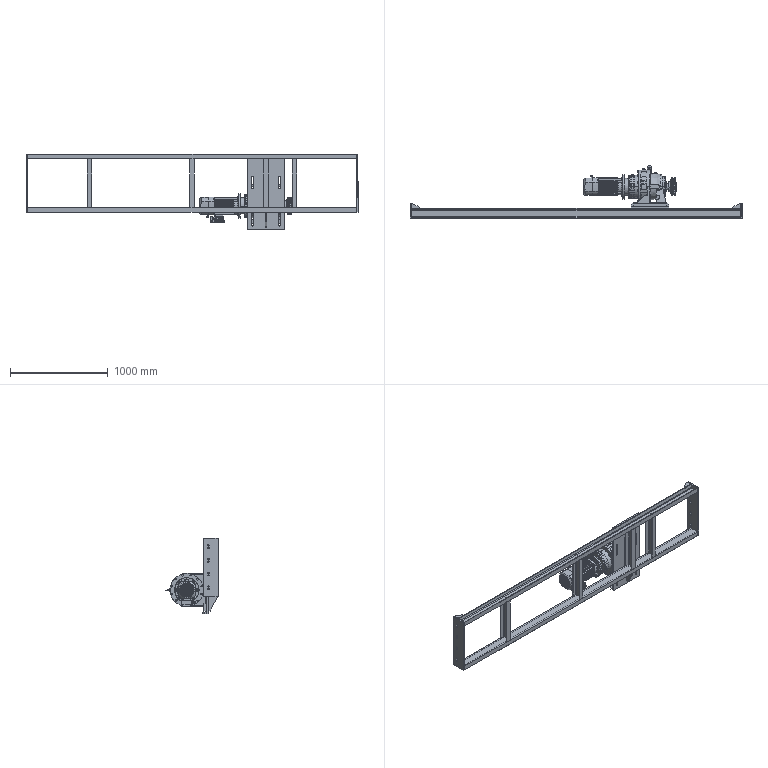Part | SolidWorks | 41 solids | 5220 faces | volume 58645223 mm3 | plane 3448 | cylinder 838 | spline 601 | cone 180 | torus 152 | sphere 1 | commonest cylinder face diameters 23.106 x90 41.467 x88 2 x71 16.059 x54 142 x47 162 x44